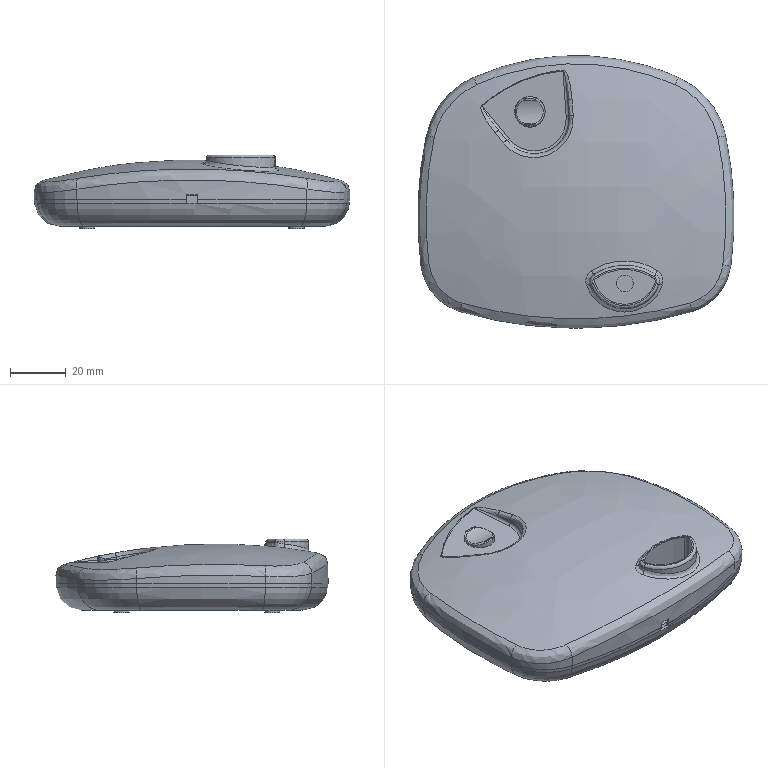Part | NX | features SKETCH 49, EXTRUDE 45, EXTRACT_DATUM_PLANE 44, EXTRACT_DATUM_AXIS 22, Instance Feature 21, BLEND 13, SIMPLE HOLE 13, DATUM_CSYS 11, HOLE PACKAGE 9, DRAFT 8, CBORE_HOLE 6, TRIMMED_SH 6, SCALE 4, SEW 3, DATUM_PLANE 2, CHAMFER 1, Pattern Feature 1, SHELL 1, SKIN 1, THICKEN_SHEET 1 | 4 solids | 418 faces | box 113.32 x 97.651 x 26.5 mm | volume 44372 mm3 | plane 188 | cylinder 111 | cone 50 | spline 39 | torus 30 | commonest cylinder face diameters 1.5 x17 3 x14 15 x8 4 x6 6 x5 2 x4